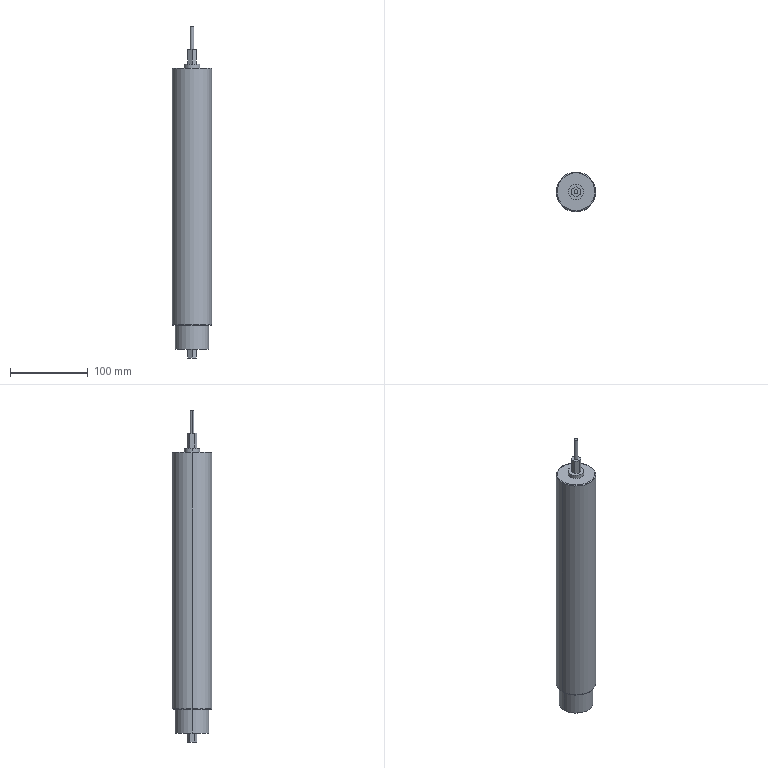Part | STEP file | Motorized Roller_Default | 1 solid | 31 faces | box 50.6 x 50.6 x 426 mm | volume 713178 mm3 | plane 19 | cylinder 8 | torus 4 | commonest cylinder face diameters 5 x2 20 x2 43 x2 50.6 x2